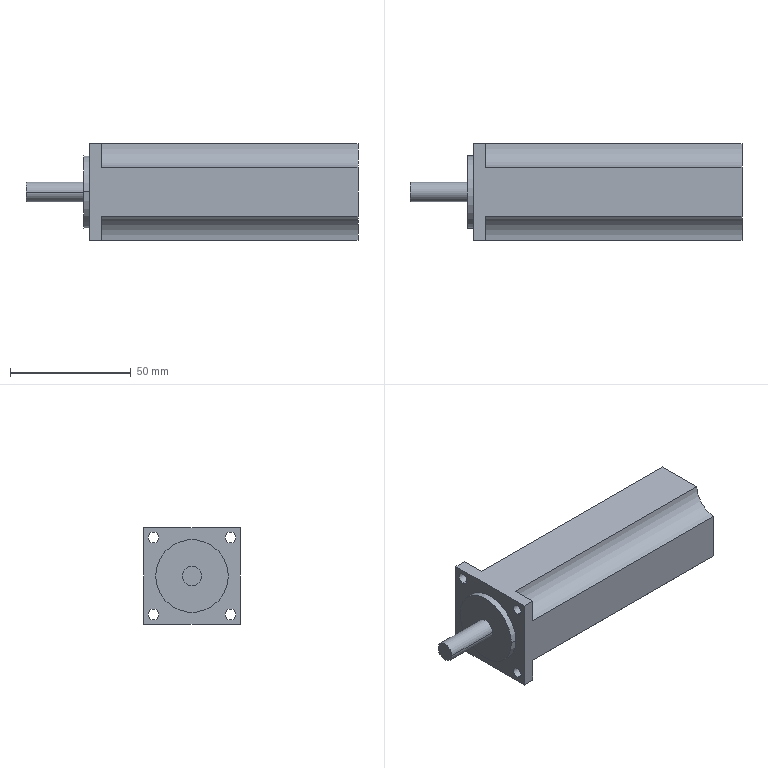Part | SolidWorks | features ICE 3, CirPattern 1, Extrusion 1, HoleWzd 1 | 1 solid | 28 faces | box 137.2 x 40 x 40 mm | volume 146758 mm3 | cylinder 16 | plane 12 | commonest cylinder face diameters 4.5 x8 20 x4 8 x2 30 x2
STEP:
#1=CARTESIAN_POINT('',(-50.4,-15.91,6.34));
#2=VERTEX_POINT('',#1);
#3=CARTESIAN_POINT('',(-50.4,-15.91,1.84));
#4=VERTEX_POINT('',#3);
#5=CARTESIAN_POINT('',(-50.4,-15.91,4.09));
#6=DIRECTION('',(1.,0.,0.));
#7=DIRECTION('',(0.,0.,-1.));
#8=AXIS2_PLACEMENT_3D('',#5,#6,#7);
#9=CIRCLE('',#8,2.25);
#10=EDGE_CURVE('',#2,#4,#9,.T.);
#11=ORIENTED_EDGE('',*,*,#10,.T.);
#12=CARTESIAN_POINT('',(-55.4,-15.91,1.84));
#13=VERTEX_POINT('',#12);
#14=CARTESIAN_POINT('',(-55.4,-15.91,1.84));
#15=DIRECTION('',(-1.,0.,0.));
#16=VECTOR('',#15,1000.);
#17=LINE('',#14,#16);
#18=EDGE_CURVE('',#4,#13,#17,.T.);
#19=ORIENTED_EDGE('',*,*,#18,.T.);
#20=CARTESIAN_POINT('',(-55.4,-15.91,6.34));
#21=VERTEX_POINT('',#20);
#22=CARTESIAN_POINT('',(-55.4,-15.91,4.09));
#23=DIRECTION('',(-1.,0.,0.));
#24=DIRECTION('',(0.,0.,1.));
#25=AXIS2_PLACEMENT_3D('',#22,#23,#24);
#26=CIRCLE('',#25,2.25);
#27=EDGE_CURVE('',#13,#21,#26,.T.);
#28=ORIENTED_EDGE('',*,*,#27,.T.);
#29=CARTESIAN_POINT('',(-55.4,-15.91,6.34));
#30=DIRECTION('',(-1.,0.,0.));
#31=VECTOR('',#30,1000.);
#32=LINE('',#29,#31);
#33=EDGE_CURVE('',#2,#21,#32,.T.);
#34=ORIENTED_EDGE('',*,*,#33,.F.);
#35=EDGE_LOOP('',(#11,#19,#28,#34));
#36=FACE_OUTER_BOUND('',#35,.T.);
#37=CARTESIAN_POINT('',(-55.4,-15.91,4.09));
#38=DIRECTION('',(-1.,0.,0.));
#39=DIRECTION('',(0.,0.,1.));
#40=AXIS2_PLACEMENT_3D('',#37,#38,#39);
#41=CYLINDRICAL_SURFACE('',#40,2.25);
#42=ADVANCED_FACE('',(#36),#41,.F.);
#43=CARTESIAN_POINT('',(-50.4,-15.91,38.16));
#44=VERTEX_POINT('',#43);
#45=CARTESIAN_POINT('',(-50.4,-15.91,33.66));
#46=VERTEX_POINT('',#45);
#47=CARTESIAN_POINT('',(-50.4,-15.91,35.91));
#48=DIRECTION('',(1.,0.,0.));
#49=DIRECTION('',(0.,0.,-1.));
#50=AXIS2_PLACEMENT_3D('',#47,#48,#49);
#51=CIRCLE('',#50,2.25);
#52=EDGE_CURVE('',#44,#46,#51,.T.);
#53=ORIENTED_EDGE('',*,*,#52,.T.);
#54=CARTESIAN_POINT('',(-55.4,-15.91,33.66));
#55=VERTEX_POINT('',#54);
#56=CARTESIAN_POINT('',(-55.4,-15.91,33.66));
#57=DIRECTION('',(-1.,0.,0.));
#58=VECTOR('',#57,1000.);
#59=LINE('',#56,#58);
#60=EDGE_CURVE('',#46,#55,#59,.T.);
#61=ORIENTED_EDGE('',*,*,#60,.T.);
#62=CARTESIAN_POINT('',(-55.4,-15.91,38.16));
#63=VERTEX_POINT('',#62);
#64=CARTESIAN_POINT('',(-55.4,-15.91,35.91));
#65=DIRECTION('',(-1.,0.,0.));
#66=DIRECTION('',(0.,0.,1.));
#67=AXIS2_PLACEMENT_3D('',#64,#65,#66);
#68=CIRCLE('',#67,2.25);
#69=EDGE_CURVE('',#55,#63,#68,.T.);
#70=ORIENTED_EDGE('',*,*,#69,.T.);
#71=CARTESIAN_POINT('',(-55.4,-15.91,38.16));
#72=DIRECTION('',(-1.,0.,0.));
#73=VECTOR('',#72,1000.);
#74=LINE('',#71,#73);
#75=EDGE_CURVE('',#44,#63,#74,.T.);
#76=ORIENTED_EDGE('',*,*,#75,.F.);
#77=EDGE_LOOP('',(#53,#61,#70,#76));
#78=FACE_OUTER_BOUND('',#77,.T.);
#79=CARTESIAN_POINT('',(-55.4,-15.91,35.91));
#80=DIRECTION('',(-1.,0.,0.));
#81=DIRECTION('',(0.,0.,1.));
#82=AXIS2_PLACEMENT_3D('',#79,#80,#81);
#83=CYLINDRICAL_SURFACE('',#82,2.25);
#84=ADVANCED_FACE('',(#78),#83,.F.);
#85=CARTESIAN_POINT('',(-50.4,15.91,38.16));
#86=VERTEX_POINT('',#85);
#87=CARTESIAN_POINT('',(-50.4,15.91,33.66));
#88=VERTEX_POINT('',#87);
#89=CARTESIAN_POINT('',(-50.4,15.91,35.91));
#90=DIRECTION('',(1.,0.,0.));
#91=DIRECTION('',(0.,0.,-1.));
#92=AXIS2_PLACEMENT_3D('',#89,#90,#91);
#93=CIRCLE('',#92,2.25);
#94=EDGE_CURVE('',#86,#88,#93,.T.);
#95=ORIENTED_EDGE('',*,*,#94,.T.);
#96=CARTESIAN_POINT('',(-55.4,15.91,33.66));
#97=VERTEX_POINT('',#96);
#98=CARTESIAN_POINT('',(-55.4,15.91,33.66));
#99=DIRECTION('',(-1.,0.,0.));
#100=VECTOR('',#99,1000.);
#101=LINE('',#98,#100);
#102=EDGE_CURVE('',#88,#97,#101,.T.);
#103=ORIENTED_EDGE('',*,*,#102,.T.);
#104=CARTESIAN_POINT('',(-55.4,15.91,38.16));
#105=VERTEX_POINT('',#104);
#106=CARTESIAN_POINT('',(-55.4,15.91,35.91));
#107=DIRECTION('',(-1.,0.,0.));
#108=DIRECTION('',(0.,0.,1.));
#109=AXIS2_PLACEMENT_3D('',#106,#107,#108);
#110=CIRCLE('',#109,2.25);
#111=EDGE_CURVE('',#97,#105,#110,.T.);
#112=ORIENTED_EDGE('',*,*,#111,.T.);
#113=CARTESIAN_POINT('',(-55.4,15.91,38.16));
#114=DIRECTION('',(-1.,0.,0.));
#115=VECTOR('',#114,1000.);
#116=LINE('',#113,#115);
#117=EDGE_CURVE('',#86,#105,#116,.T.);
#118=ORIENTED_EDGE('',*,*,#117,.F.);
#119=EDGE_LOOP('',(#95,#103,#112,#118));
#120=FACE_OUTER_BOUND('',#119,.T.);
#121=CARTESIAN_POINT('',(-55.4,15.91,35.91));
#122=DIRECTION('',(-1.,0.,0.));
#123=DIRECTION('',(0.,0.,1.));
#124=AXIS2_PLACEMENT_3D('',#121,#122,#123);
#125=CYLINDRICAL_SURFACE('',#124,2.25);
#126=ADVANCED_FACE('',(#120),#125,.F.);
#127=CARTESIAN_POINT('',(-50.4,15.91,6.34));
#128=VERTEX_POINT('',#127);
#129=CARTESIAN_POINT('',(-50.4,15.91,1.84));
#130=VERTEX_POINT('',#129);
#131=CARTESIAN_POINT('',(-50.4,15.91,4.09));
#132=DIRECTION('',(1.,0.,0.));
#133=DIRECTION('',(0.,0.,-1.));
#134=AXIS2_PLACEMENT_3D('',#131,#132,#133);
#135=CIRCLE('',#134,2.25);
#136=EDGE_CURVE('',#128,#130,#135,.T.);
#137=ORIENTED_EDGE('',*,*,#136,.T.);
#138=CARTESIAN_POINT('',(-55.4,15.91,1.84));
#139=VERTEX_POINT('',#138);
#140=CARTESIAN_POINT('',(-55.4,15.91,1.84));
#141=DIRECTION('',(-1.,0.,0.));
#142=VECTOR('',#141,1000.);
#143=LINE('',#140,#142);
#144=EDGE_CURVE('',#130,#139,#143,.T.);
#145=ORIENTED_EDGE('',*,*,#144,.T.);
#146=CARTESIAN_POINT('',(-55.4,15.91,6.34));
#147=VERTEX_POINT('',#146);
#148=CARTESIAN_POINT('',(-55.4,15.91,4.09));
#149=DIRECTION('',(-1.,0.,0.));
#150=DIRECTION('',(0.,0.,1.));
#151=AXIS2_PLACEMENT_3D('',#148,#149,#150);
#152=CIRCLE('',#151,2.25);
#153=EDGE_CURVE('',#139,#147,#152,.T.);
#154=ORIENTED_EDGE('',*,*,#153,.T.);
#155=CARTESIAN_POINT('',(-55.4,15.91,6.34));
#156=DIRECTION('',(-1.,0.,0.));
#157=VECTOR('',#156,1000.);
#158=LINE('',#155,#157);
#159=EDGE_CURVE('',#128,#147,#158,.T.);
#160=ORIENTED_EDGE('',*,*,#159,.F.);
#161=EDGE_LOOP('',(#137,#145,#154,#160));
#162=FACE_OUTER_BOUND('',#161,.T.);
#163=CARTESIAN_POINT('',(-55.4,15.91,4.09));
#164=DIRECTION('',(-1.,0.,0.));
#165=DIRECTION('',(0.,0.,1.));
#166=AXIS2_PLACEMENT_3D('',#163,#164,#165);
#167=CYLINDRICAL_SURFACE('',#166,2.25);
#168=ADVANCED_FACE('',(#162),#167,.F.);
#169=CARTESIAN_POINT('',(-81.8,-4.,20.));
#170=VERTEX_POINT('',#169);
#171=CARTESIAN_POINT('',(-81.8,4.,20.));
#172=VERTEX_POINT('',#171);
#173=CARTESIAN_POINT('',(-81.8,0.,20.));
#174=DIRECTION('',(-1.,0.,0.));
#175=DIRECTION('',(0.,-1.,0.));
#176=AXIS2_PLACEMENT_3D('',#173,#174,#175);
#177=CIRCLE('',#176,4.);
#178=EDGE_CURVE('',#170,#172,#177,.T.);
#179=ORIENTED_EDGE('',*,*,#178,.F.);
#180=CARTESIAN_POINT('',(-58.,-4.,20.));
#181=VERTEX_POINT('',#180);
#182=CARTESIAN_POINT('',(-81.8,-4.,20.));
#183=DIRECTION('',(1.,0.,0.));
#184=VECTOR('',#183,1000.);
#185=LINE('',#182,#184);
#186=EDGE_CURVE('',#170,#181,#185,.T.);
#187=ORIENTED_EDGE('',*,*,#186,.T.);
#188=CARTESIAN_POINT('',(-58.,4.,20.));
#189=VERTEX_POINT('',#188);
#190=CARTESIAN_POINT('',(-58.,0.,20.));
#191=DIRECTION('',(-1.,0.,0.));
#192=DIRECTION('',(0.,-1.,0.));
#193=AXIS2_PLACEMENT_3D('',#190,#191,#192);
#194=CIRCLE('',#193,4.);
#195=EDGE_CURVE('',#181,#189,#194,.T.);
#196=ORIENTED_EDGE('',*,*,#195,.T.);
#197=CARTESIAN_POINT('',(-81.8,4.,20.));
#198=DIRECTION('',(1.,0.,0.));
#199=VECTOR('',#198,1000.);
#200=LINE('',#197,#199);
#201=EDGE_CURVE('',#172,#189,#200,.T.);
#202=ORIENTED_EDGE('',*,*,#201,.F.);
#203=EDGE_LOOP('',(#179,#187,#196,#202));
#204=FACE_OUTER_BOUND('',#203,.T.);
#205=CARTESIAN_POINT('',(-81.8,0.,20.));
#206=DIRECTION('',(1.,0.,0.));
#207=DIRECTION('',(0.,1.,0.));
#208=AXIS2_PLACEMENT_3D('',#205,#206,#207);
#209=CYLINDRICAL_SURFACE('',#208,4.);
#210=ADVANCED_FACE('',(#204),#209,.T.);
#211=CARTESIAN_POINT('',(-58.,-15.,20.));
#212=VERTEX_POINT('',#211);
#213=CARTESIAN_POINT('',(-58.,15.,20.));
#214=VERTEX_POINT('',#213);
#215=CARTESIAN_POINT('',(-58.,0.,20.));
#216=DIRECTION('',(-1.,0.,0.));
#217=DIRECTION('',(0.,-1.,0.));
#218=AXIS2_PLACEMENT_3D('',#215,#216,#217);
#219=CIRCLE('',#218,15.);
#220=EDGE_CURVE('',#212,#214,#219,.T.);
#221=ORIENTED_EDGE('',*,*,#220,.F.);
#222=CARTESIAN_POINT('',(-55.4,-15.,20.));
#223=VERTEX_POINT('',#222);
#224=CARTESIAN_POINT('',(-58.,-15.,20.));
#225=DIRECTION('',(1.,0.,0.));
#226=VECTOR('',#225,1000.);
#227=LINE('',#224,#226);
#228=EDGE_CURVE('',#212,#223,#227,.T.);
#229=ORIENTED_EDGE('',*,*,#228,.T.);
#230=CARTESIAN_POINT('',(-55.4,15.,20.));
#231=VERTEX_POINT('',#230);
#232=CARTESIAN_POINT('',(-55.4,0.,20.));
#233=DIRECTION('',(-1.,0.,0.));
#234=DIRECTION('',(0.,1.,0.));
#235=AXIS2_PLACEMENT_3D('',#232,#233,#234);
#236=CIRCLE('',#235,15.);
#237=EDGE_CURVE('',#223,#231,#236,.T.);
#238=ORIENTED_EDGE('',*,*,#237,.T.);
#239=CARTESIAN_POINT('',(-58.,15.,20.));
#240=DIRECTION('',(1.,0.,0.));
#241=VECTOR('',#240,1000.);
#242=LINE('',#239,#241);
#243=EDGE_CURVE('',#214,#231,#242,.T.);
#244=ORIENTED_EDGE('',*,*,#243,.F.);
#245=EDGE_LOOP('',(#221,#229,#238,#244));
#246=FACE_OUTER_BOUND('',#245,.T.);
#247=CARTESIAN_POINT('',(-58.,0.,20.));
#248=DIRECTION('',(1.,0.,0.));
#249=DIRECTION('',(0.,1.,0.));
#250=AXIS2_PLACEMENT_3D('',#247,#248,#249);
#251=CYLINDRICAL_SURFACE('',#250,15.);
#252=ADVANCED_FACE('',(#246),#251,.T.);
#253=CARTESIAN_POINT('',(-58.,0.,20.));
#254=DIRECTION('',(-1.,0.,0.));
#255=DIRECTION('',(0.,-1.,0.));
#256=AXIS2_PLACEMENT_3D('',#253,#254,#255);
#257=CIRCLE('',#256,15.);
#258=EDGE_CURVE('',#214,#212,#257,.T.);
#259=ORIENTED_EDGE('',*,*,#258,.T.);
#260=ORIENTED_EDGE('',*,*,#220,.T.);
#261=EDGE_LOOP('',(#259,#260));
#262=FACE_OUTER_BOUND('',#261,.T.);
#263=CARTESIAN_POINT('',(-58.,0.,20.));
#264=DIRECTION('',(-1.,0.,0.));
#265=DIRECTION('',(0.,-1.,0.));
#266=AXIS2_PLACEMENT_3D('',#263,#264,#265);
#267=CIRCLE('',#266,4.);
#268=EDGE_CURVE('',#189,#181,#267,.T.);
#269=ORIENTED_EDGE('',*,*,#268,.F.);
#270=ORIENTED_EDGE('',*,*,#195,.F.);
#271=EDGE_LOOP('',(#269,#270));
#272=FACE_BOUND('',#271,.T.);
#273=CARTESIAN_POINT('',(-58.,0.,20.));
#274=DIRECTION('',(-1.,0.,0.));
#275=DIRECTION('',(0.,-1.,0.));
#276=AXIS2_PLACEMENT_3D('',#273,#274,#275);
#277=PLANE('',#276);
#278=ADVANCED_FACE('',(#262,#272),#277,.T.);
#279=CARTESIAN_POINT('',(-55.4,-15.91,4.09));
#280=DIRECTION('',(-1.,0.,0.));
#281=DIRECTION('',(0.,0.,1.));
#282=AXIS2_PLACEMENT_3D('',#279,#280,#281);
#283=CIRCLE('',#282,2.25);
#284=EDGE_CURVE('',#21,#13,#283,.T.);
#285=ORIENTED_EDGE('',*,*,#284,.F.);
#286=ORIENTED_EDGE('',*,*,#27,.F.);
#287=EDGE_LOOP('',(#285,#286));
#288=FACE_BOUND('',#287,.T.);
#289=CARTESIAN_POINT('',(-55.4,-15.91,35.91));
#290=DIRECTION('',(-1.,0.,0.));
#291=DIRECTION('',(0.,0.,1.));
#292=AXIS2_PLACEMENT_3D('',#289,#290,#291);
#293=CIRCLE('',#292,2.25);
#294=EDGE_CURVE('',#63,#55,#293,.T.);
#295=ORIENTED_EDGE('',*,*,#294,.F.);
#296=ORIENTED_EDGE('',*,*,#69,.F.);
#297=EDGE_LOOP('',(#295,#296));
#298=FACE_BOUND('',#297,.T.);
#299=CARTESIAN_POINT('',(-55.4,15.91,35.91));
#300=DIRECTION('',(-1.,0.,0.));
#301=DIRECTION('',(0.,0.,1.));
#302=AXIS2_PLACEMENT_3D('',#299,#300,#301);
#303=CIRCLE('',#302,2.25);
#304=EDGE_CURVE('',#105,#97,#303,.T.);
#305=ORIENTED_EDGE('',*,*,#304,.F.);
#306=ORIENTED_EDGE('',*,*,#111,.F.);
#307=EDGE_LOOP('',(#305,#306));
#308=FACE_BOUND('',#307,.T.);
#309=CARTESIAN_POINT('',(-55.4,15.91,4.09));
#310=DIRECTION('',(-1.,0.,0.));
#311=DIRECTION('',(0.,0.,1.));
#312=AXIS2_PLACEMENT_3D('',#309,#310,#311);
#313=CIRCLE('',#312,2.25);
#314=EDGE_CURVE('',#147,#139,#313,.T.);
#315=ORIENTED_EDGE('',*,*,#314,.F.);
#316=ORIENTED_EDGE('',*,*,#153,.F.);
#317=EDGE_LOOP('',(#315,#316));
#318=FACE_BOUND('',#317,.T.);
#319=CARTESIAN_POINT('',(-55.4,20.,0.));
#320=VERTEX_POINT('',#319);
#321=CARTESIAN_POINT('',(-55.4,-20.,0.));
#322=VERTEX_POINT('',#321);
#323=CARTESIAN_POINT('',(-55.4,20.,0.));
#324=DIRECTION('',(0.,-1.,0.));
#325=VECTOR('',#324,1000.);
#326=LINE('',#323,#325);
#327=EDGE_CURVE('',#320,#322,#326,.T.);
#328=ORIENTED_EDGE('',*,*,#327,.T.);
#329=CARTESIAN_POINT('',(-55.4,-20.,40.));
#330=VERTEX_POINT('',#329);
#331=CARTESIAN_POINT('',(-55.4,-20.,40.));
#332=DIRECTION('',(0.,0.,-1.));
#333=VECTOR('',#332,1000.);
#334=LINE('',#331,#333);
#335=EDGE_CURVE('',#330,#322,#334,.T.);
#336=ORIENTED_EDGE('',*,*,#335,.F.);
#337=CARTESIAN_POINT('',(-55.4,20.,40.));
#338=VERTEX_POINT('',#337);
#339=CARTESIAN_POINT('',(-55.4,20.,40.));
#340=DIRECTION('',(0.,-1.,0.));
#341=VECTOR('',#340,1000.);
#342=LINE('',#339,#341);
#343=EDGE_CURVE('',#338,#330,#342,.T.);
#344=ORIENTED_EDGE('',*,*,#343,.F.);
#345=CARTESIAN_POINT('',(-55.4,20.,40.));
#346=DIRECTION('',(0.,0.,-1.));
#347=VECTOR('',#346,1000.);
#348=LINE('',#345,#347);
#349=EDGE_CURVE('',#338,#320,#348,.T.);
#350=ORIENTED_EDGE('',*,*,#349,.T.);
#351=EDGE_LOOP('',(#328,#336,#344,#350));
#352=FACE_OUTER_BOUND('',#351,.T.);
#353=CARTESIAN_POINT('',(-55.4,0.,20.));
#354=DIRECTION('',(-1.,0.,0.));
#355=DIRECTION('',(0.,1.,0.));
#356=AXIS2_PLACEMENT_3D('',#353,#354,#355);
#357=CIRCLE('',#356,15.);
#358=EDGE_CURVE('',#231,#223,#357,.T.);
#359=ORIENTED_EDGE('',*,*,#358,.F.);
#360=ORIENTED_EDGE('',*,*,#237,.F.);
#361=EDGE_LOOP('',(#359,#360));
#362=FACE_BOUND('',#361,.T.);
#363=CARTESIAN_POINT('',(-55.4,20.,40.));
#364=DIRECTION('',(1.,0.,0.));
#365=DIRECTION('',(0.,1.,0.));
#366=AXIS2_PLACEMENT_3D('',#363,#364,#365);
#367=PLANE('',#366);
#368=ADVANCED_FACE('',(#288,#298,#308,#318,#352,#362),#367,.F.);
#369=CARTESIAN_POINT('',(55.4,-20.,30.));
#370=VERTEX_POINT('',#369);
#371=CARTESIAN_POINT('',(55.4,-20.,10.));
#372=VERTEX_POINT('',#371);
#373=CARTESIAN_POINT('',(55.4,-20.,40.));
#374=DIRECTION('',(0.,0.,-1.));
#375=VECTOR('',#374,1000.);
#376=LINE('',#373,#375);
#377=EDGE_CURVE('',#370,#372,#376,.T.);
#378=ORIENTED_EDGE('',*,*,#377,.T.);
#379=CARTESIAN_POINT('',(55.4,-10.,0.));
#380=VERTEX_POINT('',#379);
#381=CARTESIAN_POINT('',(55.4,-20.,0.));
#382=DIRECTION('',(1.,0.,0.));
#383=DIRECTION('',(0.,0.,-1.));
#384=AXIS2_PLACEMENT_3D('',#381,#382,#383);
#385=CIRCLE('',#384,10.);
#386=EDGE_CURVE('',#380,#372,#385,.T.);
#387=ORIENTED_EDGE('',*,*,#386,.F.);
#388=CARTESIAN_POINT('',(55.4,10.,0.));
#389=VERTEX_POINT('',#388);
#390=CARTESIAN_POINT('',(55.4,20.,0.));
#391=DIRECTION('',(0.,1.,0.));
#392=VECTOR('',#391,1000.);
#393=LINE('',#390,#392);
#394=EDGE_CURVE('',#380,#389,#393,.T.);
#395=ORIENTED_EDGE('',*,*,#394,.T.);
#396=CARTESIAN_POINT('',(55.4,20.,10.));
#397=VERTEX_POINT('',#396);
#398=CARTESIAN_POINT('',(55.4,20.,0.));
#399=DIRECTION('',(1.,0.,0.));
#400=DIRECTION('',(0.,0.,-1.));
#401=AXIS2_PLACEMENT_3D('',#398,#399,#400);
#402=CIRCLE('',#401,10.);
#403=EDGE_CURVE('',#397,#389,#402,.T.);
#404=ORIENTED_EDGE('',*,*,#403,.F.);
#405=CARTESIAN_POINT('',(55.4,20.,30.));
#406=VERTEX_POINT('',#405);
#407=CARTESIAN_POINT('',(55.4,20.,40.));
#408=DIRECTION('',(0.,0.,-1.));
#409=VECTOR('',#408,1000.);
#410=LINE('',#407,#409);
#411=EDGE_CURVE('',#406,#397,#410,.T.);
#412=ORIENTED_EDGE('',*,*,#411,.F.);
#413=CARTESIAN_POINT('',(55.4,10.,40.));
#414=VERTEX_POINT('',#413);
#415=CARTESIAN_POINT('',(55.4,20.,40.));
#416=DIRECTION('',(1.,0.,0.));
#417=DIRECTION('',(0.,0.,-1.));
#418=AXIS2_PLACEMENT_3D('',#415,#416,#417);
#419=CIRCLE('',#418,10.);
#420=EDGE_CURVE('',#414,#406,#419,.T.);
#421=ORIENTED_EDGE('',*,*,#420,.F.);
#422=CARTESIAN_POINT('',(55.4,-10.,40.));
#423=VERTEX_POINT('',#422);
#424=CARTESIAN_POINT('',(55.4,20.,40.));
#425=DIRECTION('',(0.,1.,0.));
#426=VECTOR('',#425,1000.);
#427=LINE('',#424,#426);
#428=EDGE_CURVE('',#423,#414,#427,.T.);
#429=ORIENTED_EDGE('',*,*,#428,.F.);
#430=CARTESIAN_POINT('',(55.4,-20.,40.));
#431=DIRECTION('',(1.,0.,0.));
#432=DIRECTION('',(0.,0.,-1.));
#433=AXIS2_PLACEMENT_3D('',#430,#431,#432);
#434=CIRCLE('',#433,10.);
#435=EDGE_CURVE('',#370,#423,#434,.T.);
#436=ORIENTED_EDGE('',*,*,#435,.F.);
#437=EDGE_LOOP('',(#378,#387,#395,#404,#412,#421,#429,#436));
#438=FACE_OUTER_BOUND('',#437,.T.);
#439=CARTESIAN_POINT('',(55.4,20.,40.));
#440=DIRECTION('',(-1.,0.,0.));
#441=DIRECTION('',(0.,0.,1.));
#442=AXIS2_PLACEMENT_3D('',#439,#440,#441);
#443=PLANE('',#442);
#444=ADVANCED_FACE('',(#438),#443,.F.);
#445=ORIENTED_EDGE('',*,*,#411,.T.);
#446=CARTESIAN_POINT('',(-50.4,20.,10.));
#447=VERTEX_POINT('',#446);
#448=CARTESIAN_POINT('',(-50.4,20.,10.));
#449=DIRECTION('',(-1.,0.,0.));
#450=VECTOR('',#449,1000.);
#451=LINE('',#448,#450);
#452=EDGE_CURVE('',#397,#447,#451,.T.);
#453=ORIENTED_EDGE('',*,*,#452,.T.);
#454=CARTESIAN_POINT('',(-50.4,20.,0.));
#455=VERTEX_POINT('',#454);
#456=CARTESIAN_POINT('',(-50.4,20.,40.));
#457=DIRECTION('',(0.,0.,1.));
#458=VECTOR('',#457,1000.);
#459=LINE('',#456,#458);
#460=EDGE_CURVE('',#455,#447,#459,.T.);
#461=ORIENTED_EDGE('',*,*,#460,.F.);
#462=CARTESIAN_POINT('',(-55.4,20.,0.));
#463=DIRECTION('',(-1.,0.,0.));
#464=VECTOR('',#463,1000.);
#465=LINE('',#462,#464);
#466=EDGE_CURVE('',#455,#320,#465,.T.);
#467=ORIENTED_EDGE('',*,*,#466,.T.);
#468=ORIENTED_EDGE('',*,*,#349,.F.);
#469=CARTESIAN_POINT('',(-50.4,20.,40.));
#470=VERTEX_POINT('',#469);
#471=CARTESIAN_POINT('',(-55.4,20.,40.));
#472=DIRECTION('',(-1.,0.,0.));
#473=VECTOR('',#472,1000.);
#474=LINE('',#471,#473);
#475=EDGE_CURVE('',#470,#338,#474,.T.);
#476=ORIENTED_EDGE('',*,*,#475,.F.);
#477=CARTESIAN_POINT('',(-50.4,20.,30.));
#478=VERTEX_POINT('',#477);
#479=CARTESIAN_POINT('',(-50.4,20.,40.));
#480=DIRECTION('',(0.,0.,1.));
#481=VECTOR('',#480,1000.);
#482=LINE('',#479,#481);
#483=EDGE_CURVE('',#478,#470,#482,.T.);
#484=ORIENTED_EDGE('',*,*,#483,.F.);
#485=CARTESIAN_POINT('',(-50.4,20.,30.));
#486=DIRECTION('',(1.,0.,0.));
#487=VECTOR('',#486,1000.);
#488=LINE('',#485,#487);
#489=EDGE_CURVE('',#478,#406,#488,.T.);
#490=ORIENTED_EDGE('',*,*,#489,.T.);
#491=EDGE_LOOP('',(#445,#453,#461,#467,#468,#476,#484,#490));
#492=FACE_OUTER_BOUND('',#491,.T.);
#493=CARTESIAN_POINT('',(-55.4,20.,40.));
#494=DIRECTION('',(0.,-1.,0.));
#495=DIRECTION('',(0.,0.,-1.));
#496=AXIS2_PLACEMENT_3D('',#493,#494,#495);
#497=PLANE('',#496);
#498=ADVANCED_FACE('',(#492),#497,.F.);
#499=CARTESIAN_POINT('',(-50.4,-20.,10.));
#500=VERTEX_POINT('',#499);
#501=CARTESIAN_POINT('',(-50.4,-20.,0.));
#502=VERTEX_POINT('',#501);
#503=CARTESIAN_POINT('',(-50.4,-20.,40.));
#504=DIRECTION('',(0.,0.,-1.));
#505=VECTOR('',#504,1000.);
#506=LINE('',#503,#505);
#507=EDGE_CURVE('',#500,#502,#506,.T.);
#508=ORIENTED_EDGE('',*,*,#507,.F.);
#509=CARTESIAN_POINT('',(-50.4,-20.,10.));
#510=DIRECTION('',(1.,0.,0.));
#511=VECTOR('',#510,1000.);
#512=LINE('',#509,#511);
#513=EDGE_CURVE('',#500,#372,#512,.T.);
#514=ORIENTED_EDGE('',*,*,#513,.T.);
#515=ORIENTED_EDGE('',*,*,#377,.F.);
#516=CARTESIAN_POINT('',(-50.4,-20.,30.));
#517=VERTEX_POINT('',#516);
#518=CARTESIAN_POINT('',(-50.4,-20.,30.));
#519=DIRECTION('',(-1.,0.,0.));
#520=VECTOR('',#519,1000.);
#521=LINE('',#518,#520);
#522=EDGE_CURVE('',#370,#517,#521,.T.);
#523=ORIENTED_EDGE('',*,*,#522,.T.);
#524=CARTESIAN_POINT('',(-50.4,-20.,40.));
#525=VERTEX_POINT('',#524);
#526=CARTESIAN_POINT('',(-50.4,-20.,40.));
#527=DIRECTION('',(0.,0.,-1.));
#528=VECTOR('',#527,1000.);
#529=LINE('',#526,#528);
#530=EDGE_CURVE('',#525,#517,#529,.T.);
#531=ORIENTED_EDGE('',*,*,#530,.F.);
#532=CARTESIAN_POINT('',(-55.4,-20.,40.));
#533=DIRECTION('',(1.,0.,0.));
#534=VECTOR('',#533,1000.);
#535=LINE('',#532,#534);
#536=EDGE_CURVE('',#330,#525,#535,.T.);
#537=ORIENTED_EDGE('',*,*,#536,.F.);
#538=ORIENTED_EDGE('',*,*,#335,.T.);
#539=CARTESIAN_POINT('',(-55.4,-20.,0.));
#540=DIRECTION('',(1.,0.,0.));
#541=VECTOR('',#540,1000.);
#542=LINE('',#539,#541);
#543=EDGE_CURVE('',#322,#502,#542,.T.);
#544=ORIENTED_EDGE('',*,*,#543,.T.);
#545=EDGE_LOOP('',(#508,#514,#515,#523,#531,#537,#538,#544));
#546=FACE_OUTER_BOUND('',#545,.T.);
#547=CARTESIAN_POINT('',(-55.4,-20.,40.));
#548=DIRECTION('',(0.,1.,0.));
#549=DIRECTION('',(0.,0.,1.));
#550=AXIS2_PLACEMENT_3D('',#547,#548,#549);
#551=PLANE('',#550);
#552=ADVANCED_FACE('',(#546),#551,.F.);
#553=CARTESIAN_POINT('',(-50.4,-10.,40.));
#554=VERTEX_POINT('',#553);
#555=CARTESIAN_POINT('',(-50.4,-10.,40.));
#556=DIRECTION('',(-1.,0.,0.));
#557=VECTOR('',#556,1000.);
#558=LINE('',#555,#557);
#559=EDGE_CURVE('',#423,#554,#558,.T.);
#560=ORIENTED_EDGE('',*,*,#559,.F.);
#561=ORIENTED_EDGE('',*,*,#428,.T.);
#562=CARTESIAN_POINT('',(-50.4,10.,40.));
#563=VERTEX_POINT('',#562);
#564=CARTESIAN_POINT('',(-50.4,10.,40.));
#565=DIRECTION('',(1.,0.,0.));
#566=VECTOR('',#565,1000.);
#567=LINE('',#564,#566);
#568=EDGE_CURVE('',#563,#414,#567,.T.);
#569=ORIENTED_EDGE('',*,*,#568,.F.);
#570=CARTESIAN_POINT('',(-50.4,0.,40.));
#571=DIRECTION('',(0.,1.,0.));
#572=VECTOR('',#571,1000.);
#573=LINE('',#570,#572);
#574=EDGE_CURVE('',#563,#470,#573,.T.);
#575=ORIENTED_EDGE('',*,*,#574,.T.);
#576=ORIENTED_EDGE('',*,*,#475,.T.);
#577=ORIENTED_EDGE('',*,*,#343,.T.);
#578=ORIENTED_EDGE('',*,*,#536,.T.);
#579=CARTESIAN_POINT('',(-50.4,0.,40.));
#580=DIRECTION('',(0.,1.,0.));
#581=VECTOR('',#580,1000.);
#582=LINE('',#579,#581);
#583=EDGE_CURVE('',#525,#554,#582,.T.);
#584=ORIENTED_EDGE('',*,*,#583,.T.);
#585=EDGE_LOOP('',(#560,#561,#569,#575,#576,#577,#578,#584));
#586=FACE_OUTER_BOUND('',#585,.T.);
#587=CARTESIAN_POINT('',(0.,0.,40.));
#588=DIRECTION('',(0.,0.,1.));
#589=DIRECTION('',(1.,0.,0.));
#590=AXIS2_PLACEMENT_3D('',#587,#588,#589);
#591=PLANE('',#590);
#592=ADVANCED_FACE('',(#586),#591,.T.);
#593=ORIENTED_EDGE('',*,*,#394,.F.);
#594=CARTESIAN_POINT('',(-50.4,-10.,0.));
#595=VERTEX_POINT('',#594);
#596=CARTESIAN_POINT('',(-50.4,-10.,0.));
#597=DIRECTION('',(-1.,0.,0.));
#598=VECTOR('',#597,1000.);
#599=LINE('',#596,#598);
#600=EDGE_CURVE('',#380,#595,#599,.T.);
#601=ORIENTED_EDGE('',*,*,#600,.T.);
#602=CARTESIAN_POINT('',(-50.4,0.,0.));
#603=DIRECTION('',(0.,1.,0.));
#604=VECTOR('',#603,1000.);
#605=LINE('',#602,#604);
#606=EDGE_CURVE('',#502,#595,#605,.T.);
#607=ORIENTED_EDGE('',*,*,#606,.F.);
#608=ORIENTED_EDGE('',*,*,#543,.F.);
#609=ORIENTED_EDGE('',*,*,#327,.F.);
#610=ORIENTED_EDGE('',*,*,#466,.F.);
#611=CARTESIAN_POINT('',(-50.4,10.,0.));
#612=VERTEX_POINT('',#611);
#613=CARTESIAN_POINT('',(-50.4,0.,0.));
#614=DIRECTION('',(0.,1.,0.));
#615=VECTOR('',#614,1000.);
#616=LINE('',#613,#615);
#617=EDGE_CURVE('',#612,#455,#616,.T.);
#618=ORIENTED_EDGE('',*,*,#617,.F.);
#619=CARTESIAN_POINT('',(-50.4,10.,0.));
#620=DIRECTION('',(1.,0.,0.));
#621=VECTOR('',#620,1000.);
#622=LINE('',#619,#621);
#623=EDGE_CURVE('',#612,#389,#622,.T.);
#624=ORIENTED_EDGE('',*,*,#623,.T.);
#625=EDGE_LOOP('',(#593,#601,#607,#608,#609,#610,#618,#624));
#626=FACE_OUTER_BOUND('',#625,.T.);
#627=CARTESIAN_POINT('',(0.,0.,0.));
#628=DIRECTION('',(0.,0.,1.));
#629=DIRECTION('',(1.,0.,0.));
#630=AXIS2_PLACEMENT_3D('',#627,#628,#629);
#631=PLANE('',#630);
#632=ADVANCED_FACE('',(#626),#631,.F.);
#633=ORIENTED_EDGE('',*,*,#228,.F.);
#634=ORIENTED_EDGE('',*,*,#258,.F.);
#635=ORIENTED_EDGE('',*,*,#243,.T.);
#636=ORIENTED_EDGE('',*,*,#358,.T.);
#637=EDGE_LOOP('',(#633,#634,#635,#636));
#638=FACE_OUTER_BOUND('',#637,.T.);
#639=CARTESIAN_POINT('',(-58.,0.,20.));
#640=DIRECTION('',(1.,0.,0.));
#641=DIRECTION('',(0.,1.,0.));
#642=AXIS2_PLACEMENT_3D('',#639,#640,#641);
#643=CYLINDRICAL_SURFACE('',#642,15.);
#644=ADVANCED_FACE('',(#638),#643,.T.);
#645=ORIENTED_EDGE('',*,*,#186,.F.);
#646=CARTESIAN_POINT('',(-81.8,0.,20.));
#647=DIRECTION('',(-1.,0.,0.));
#648=DIRECTION('',(0.,-1.,0.));
#649=AXIS2_PLACEMENT_3D('',#646,#647,#648);
#650=CIRCLE('',#649,4.);
#651=EDGE_CURVE('',#172,#170,#650,.T.);
#652=ORIENTED_EDGE('',*,*,#651,.F.);
#653=ORIENTED_EDGE('',*,*,#201,.T.);
#654=ORIENTED_EDGE('',*,*,#268,.T.);
#655=EDGE_LOOP('',(#645,#652,#653,#654));
#656=FACE_OUTER_BOUND('',#655,.T.);
#657=CARTESIAN_POINT('',(-81.8,0.,20.));
#658=DIRECTION('',(1.,0.,0.));
#659=DIRECTION('',(0.,1.,0.));
#660=AXIS2_PLACEMENT_3D('',#657,#658,#659);
#661=CYLINDRICAL_SURFACE('',#660,4.);
#662=ADVANCED_FACE('',(#656),#661,.T.);
#663=ORIENTED_EDGE('',*,*,#651,.T.);
#664=ORIENTED_EDGE('',*,*,#178,.T.);
#665=EDGE_LOOP('',(#663,#664));
#666=FACE_OUTER_BOUND('',#665,.T.);
#667=CARTESIAN_POINT('',(-81.8,0.,20.));
#668=DIRECTION('',(-1.,0.,0.));
#669=DIRECTION('',(0.,-1.,0.));
#670=AXIS2_PLACEMENT_3D('',#667,#668,#669);
#671=PLANE('',#670);
#672=ADVANCED_FACE('',(#666),#671,.T.);
#673=CARTESIAN_POINT('',(-50.4,20.,40.));
#674=DIRECTION('',(1.,0.,0.));
#675=DIRECTION('',(0.,0.,-1.));
#676=AXIS2_PLACEMENT_3D('',#673,#674,#675);
#677=CIRCLE('',#676,10.);
#678=EDGE_CURVE('',#563,#478,#677,.T.);
#679=ORIENTED_EDGE('',*,*,#678,.F.);
#680=ORIENTED_EDGE('',*,*,#568,.T.);
#681=ORIENTED_EDGE('',*,*,#420,.T.);
#682=ORIENTED_EDGE('',*,*,#489,.F.);
#683=EDGE_LOOP('',(#679,#680,#681,#682));
#684=FACE_OUTER_BOUND('',#683,.T.);
#685=CARTESIAN_POINT('',(-50.4,20.,40.));
#686=DIRECTION('',(1.,0.,0.));
#687=DIRECTION('',(0.,0.,-1.));
#688=AXIS2_PLACEMENT_3D('',#685,#686,#687);
#689=CYLINDRICAL_SURFACE('',#688,10.);
#690=ADVANCED_FACE('',(#684),#689,.F.);
#691=ORIENTED_EDGE('',*,*,#94,.F.);
#692=CARTESIAN_POINT('',(-50.4,15.91,35.91));
#693=DIRECTION('',(1.,0.,0.));
#694=DIRECTION('',(0.,0.,-1.));
#695=AXIS2_PLACEMENT_3D('',#692,#693,#694);
#696=CIRCLE('',#695,2.25);
#697=EDGE_CURVE('',#88,#86,#696,.T.);
#698=ORIENTED_EDGE('',*,*,#697,.F.);
#699=EDGE_LOOP('',(#691,#698));
#700=FACE_BOUND('',#699,.T.);
#701=ORIENTED_EDGE('',*,*,#483,.T.);
#702=ORIENTED_EDGE('',*,*,#574,.F.);
#703=ORIENTED_EDGE('',*,*,#678,.T.);
#704=EDGE_LOOP('',(#701,#702,#703));
#705=FACE_OUTER_BOUND('',#704,.T.);
#706=CARTESIAN_POINT('',(-50.4,20.,40.));
#707=DIRECTION('',(1.,0.,0.));
#708=DIRECTION('',(0.,0.,-1.));
#709=AXIS2_PLACEMENT_3D('',#706,#707,#708);
#710=PLANE('',#709);
#711=ADVANCED_FACE('',(#700,#705),#710,.T.);
#712=ORIENTED_EDGE('',*,*,#403,.T.);
#713=ORIENTED_EDGE('',*,*,#623,.F.);
#714=CARTESIAN_POINT('',(-50.4,20.,0.));
#715=DIRECTION('',(1.,0.,0.));
#716=DIRECTION('',(0.,0.,-1.));
#717=AXIS2_PLACEMENT_3D('',#714,#715,#716);
#718=CIRCLE('',#717,10.);
#719=EDGE_CURVE('',#447,#612,#718,.T.);
#720=ORIENTED_EDGE('',*,*,#719,.F.);
#721=ORIENTED_EDGE('',*,*,#452,.F.);
#722=EDGE_LOOP('',(#712,#713,#720,#721));
#723=FACE_OUTER_BOUND('',#722,.T.);
#724=CARTESIAN_POINT('',(-50.4,20.,0.));
#725=DIRECTION('',(1.,0.,0.));
#726=DIRECTION('',(0.,0.,-1.));
#727=AXIS2_PLACEMENT_3D('',#724,#725,#726);
#728=CYLINDRICAL_SURFACE('',#727,10.);
#729=ADVANCED_FACE('',(#723),#728,.F.);
#730=ORIENTED_EDGE('',*,*,#136,.F.);
#731=CARTESIAN_POINT('',(-50.4,15.91,4.09));
#732=DIRECTION('',(1.,0.,0.));
#733=DIRECTION('',(0.,0.,-1.));
#734=AXIS2_PLACEMENT_3D('',#731,#732,#733);
#735=CIRCLE('',#734,2.25);
#736=EDGE_CURVE('',#130,#128,#735,.T.);
#737=ORIENTED_EDGE('',*,*,#736,.F.);
#738=EDGE_LOOP('',(#730,#737));
#739=FACE_BOUND('',#738,.T.);
#740=ORIENTED_EDGE('',*,*,#460,.T.);
#741=ORIENTED_EDGE('',*,*,#719,.T.);
#742=ORIENTED_EDGE('',*,*,#617,.T.);
#743=EDGE_LOOP('',(#740,#741,#742));
#744=FACE_OUTER_BOUND('',#743,.T.);
#745=CARTESIAN_POINT('',(-50.4,20.,0.));
#746=DIRECTION('',(1.,0.,0.));
#747=DIRECTION('',(0.,0.,-1.));
#748=AXIS2_PLACEMENT_3D('',#745,#746,#747);
#749=PLANE('',#748);
#750=ADVANCED_FACE('',(#739,#744),#749,.T.);
#751=ORIENTED_EDGE('',*,*,#435,.T.);
#752=ORIENTED_EDGE('',*,*,#559,.T.);
#753=CARTESIAN_POINT('',(-50.4,-20.,40.));
#754=DIRECTION('',(1.,0.,0.));
#755=DIRECTION('',(0.,0.,-1.));
#756=AXIS2_PLACEMENT_3D('',#753,#754,#755);
#757=CIRCLE('',#756,10.);
#758=EDGE_CURVE('',#517,#554,#757,.T.);
#759=ORIENTED_EDGE('',*,*,#758,.F.);
#760=ORIENTED_EDGE('',*,*,#522,.F.);
#761=EDGE_LOOP('',(#751,#752,#759,#760));
#762=FACE_OUTER_BOUND('',#761,.T.);
#763=CARTESIAN_POINT('',(-50.4,-20.,40.));
#764=DIRECTION('',(1.,0.,0.));
#765=DIRECTION('',(0.,0.,-1.));
#766=AXIS2_PLACEMENT_3D('',#763,#764,#765);
#767=CYLINDRICAL_SURFACE('',#766,10.);
#768=ADVANCED_FACE('',(#762),#767,.F.);
#769=ORIENTED_EDGE('',*,*,#52,.F.);
#770=CARTESIAN_POINT('',(-50.4,-15.91,35.91));
#771=DIRECTION('',(1.,0.,0.));
#772=DIRECTION('',(0.,0.,-1.));
#773=AXIS2_PLACEMENT_3D('',#770,#771,#772);
#774=CIRCLE('',#773,2.25);
#775=EDGE_CURVE('',#46,#44,#774,.T.);
#776=ORIENTED_EDGE('',*,*,#775,.F.);
#777=EDGE_LOOP('',(#769,#776));
#778=FACE_BOUND('',#777,.T.);
#779=ORIENTED_EDGE('',*,*,#530,.T.);
#780=ORIENTED_EDGE('',*,*,#758,.T.);
#781=ORIENTED_EDGE('',*,*,#583,.F.);
#782=EDGE_LOOP('',(#779,#780,#781));
#783=FACE_OUTER_BOUND('',#782,.T.);
#784=CARTESIAN_POINT('',(-50.4,-20.,40.));
#785=DIRECTION('',(1.,0.,0.));
#786=DIRECTION('',(0.,0.,-1.));
#787=AXIS2_PLACEMENT_3D('',#784,#785,#786);
#788=PLANE('',#787);
#789=ADVANCED_FACE('',(#778,#783),#788,.T.);
#790=CARTESIAN_POINT('',(-50.4,-20.,0.));
#791=DIRECTION('',(1.,0.,0.));
#792=DIRECTION('',(0.,0.,-1.));
#793=AXIS2_PLACEMENT_3D('',#790,#791,#792);
#794=CIRCLE('',#793,10.);
#795=EDGE_CURVE('',#595,#500,#794,.T.);
#796=ORIENTED_EDGE('',*,*,#795,.F.);
#797=ORIENTED_EDGE('',*,*,#600,.F.);
#798=ORIENTED_EDGE('',*,*,#386,.T.);
#799=ORIENTED_EDGE('',*,*,#513,.F.);
#800=EDGE_LOOP('',(#796,#797,#798,#799));
#801=FACE_OUTER_BOUND('',#800,.T.);
#802=CARTESIAN_POINT('',(-50.4,-20.,0.));
#803=DIRECTION('',(1.,0.,0.));
#804=DIRECTION('',(0.,0.,-1.));
#805=AXIS2_PLACEMENT_3D('',#802,#803,#804);
#806=CYLINDRICAL_SURFACE('',#805,10.);
#807=ADVANCED_FACE('',(#801),#806,.F.);
#808=ORIENTED_EDGE('',*,*,#10,.F.);
#809=CARTESIAN_POINT('',(-50.4,-15.91,4.09));
#810=DIRECTION('',(1.,0.,0.));
#811=DIRECTION('',(0.,0.,-1.));
#812=AXIS2_PLACEMENT_3D('',#809,#810,#811);
#813=CIRCLE('',#812,2.25);
#814=EDGE_CURVE('',#4,#2,#813,.T.);
#815=ORIENTED_EDGE('',*,*,#814,.F.);
#816=EDGE_LOOP('',(#808,#815));
#817=FACE_BOUND('',#816,.T.);
#818=ORIENTED_EDGE('',*,*,#507,.T.);
#819=ORIENTED_EDGE('',*,*,#606,.T.);
#820=ORIENTED_EDGE('',*,*,#795,.T.);
#821=EDGE_LOOP('',(#818,#819,#820));
#822=FACE_OUTER_BOUND('',#821,.T.);
#823=CARTESIAN_POINT('',(-50.4,-20.,0.));
#824=DIRECTION('',(1.,0.,0.));
#825=DIRECTION('',(0.,0.,-1.));
#826=AXIS2_PLACEMENT_3D('',#823,#824,#825);
#827=PLANE('',#826);
#828=ADVANCED_FACE('',(#817,#822),#827,.T.);
#829=ORIENTED_EDGE('',*,*,#144,.F.);
#830=ORIENTED_EDGE('',*,*,#736,.T.);
#831=ORIENTED_EDGE('',*,*,#159,.T.);
#832=ORIENTED_EDGE('',*,*,#314,.T.);
#833=EDGE_LOOP('',(#829,#830,#831,#832));
#834=FACE_OUTER_BOUND('',#833,.T.);
#835=CARTESIAN_POINT('',(-55.4,15.91,4.09));
#836=DIRECTION('',(-1.,0.,0.));
#837=DIRECTION('',(0.,0.,1.));
#838=AXIS2_PLACEMENT_3D('',#835,#836,#837);
#839=CYLINDRICAL_SURFACE('',#838,2.25);
#840=ADVANCED_FACE('',(#834),#839,.F.);
#841=ORIENTED_EDGE('',*,*,#102,.F.);
#842=ORIENTED_EDGE('',*,*,#697,.T.);
#843=ORIENTED_EDGE('',*,*,#117,.T.);
#844=ORIENTED_EDGE('',*,*,#304,.T.);
#845=EDGE_LOOP('',(#841,#842,#843,#844));
#846=FACE_OUTER_BOUND('',#845,.T.);
#847=CARTESIAN_POINT('',(-55.4,15.91,35.91));
#848=DIRECTION('',(-1.,0.,0.));
#849=DIRECTION('',(0.,0.,1.));
#850=AXIS2_PLACEMENT_3D('',#847,#848,#849);
#851=CYLINDRICAL_SURFACE('',#850,2.25);
#852=ADVANCED_FACE('',(#846),#851,.F.);
#853=ORIENTED_EDGE('',*,*,#60,.F.);
#854=ORIENTED_EDGE('',*,*,#775,.T.);
#855=ORIENTED_EDGE('',*,*,#75,.T.);
#856=ORIENTED_EDGE('',*,*,#294,.T.);
#857=EDGE_LOOP('',(#853,#854,#855,#856));
#858=FACE_OUTER_BOUND('',#857,.T.);
#859=CARTESIAN_POINT('',(-55.4,-15.91,35.91));
#860=DIRECTION('',(-1.,0.,0.));
#861=DIRECTION('',(0.,0.,1.));
#862=AXIS2_PLACEMENT_3D('',#859,#860,#861);
#863=CYLINDRICAL_SURFACE('',#862,2.25);
#864=ADVANCED_FACE('',(#858),#863,.F.);
#865=ORIENTED_EDGE('',*,*,#18,.F.);
#866=ORIENTED_EDGE('',*,*,#814,.T.);
#867=ORIENTED_EDGE('',*,*,#33,.T.);
#868=ORIENTED_EDGE('',*,*,#284,.T.);
#869=EDGE_LOOP('',(#865,#866,#867,#868));
#870=FACE_OUTER_BOUND('',#869,.T.);
#871=CARTESIAN_POINT('',(-55.4,-15.91,4.09));
#872=DIRECTION('',(-1.,0.,0.));
#873=DIRECTION('',(0.,0.,1.));
#874=AXIS2_PLACEMENT_3D('',#871,#872,#873);
#875=CYLINDRICAL_SURFACE('',#874,2.25);
#876=ADVANCED_FACE('',(#870),#875,.F.);
#877=CLOSED_SHELL('',(#42,#84,#126,#168,#210,#252,#278,#368,#444,#498,#552,#592,#632,#644,#662,#672,#690,#711,#729,#750,#768,#789,#807,#828,#840,#852,#864,#876));
#878=MANIFOLD_SOLID_BREP('',#877);
#879=CARTESIAN_POINT('',(0.,0.,0.));
#880=DIRECTION('',(0.,0.,1.));
#881=DIRECTION('',(1.,0.,0.));
#882=AXIS2_PLACEMENT_3D('',#879,#880,#881);
#883=(LENGTH_UNIT()NAMED_UNIT(*)SI_UNIT(.MILLI.,.METRE.));
#884=UNCERTAINTY_MEASURE_WITH_UNIT(LENGTH_MEASURE(0.00001),#883,'','');
#885=(NAMED_UNIT(*)PLANE_ANGLE_UNIT()SI_UNIT($,.RADIAN.));
#886=(NAMED_UNIT(*)SI_UNIT($,.STERADIAN.)SOLID_ANGLE_UNIT());
#887=(GEOMETRIC_REPRESENTATION_CONTEXT(3)GLOBAL_UNCERTAINTY_ASSIGNED_CONTEXT((#884))GLOBAL_UNIT_ASSIGNED_CONTEXT((#883,#885,#886))REPRESENTATION_CONTEXT('',''));
#888=ADVANCED_BREP_SHAPE_REPRESENTATION('',(#878,#882),#887);